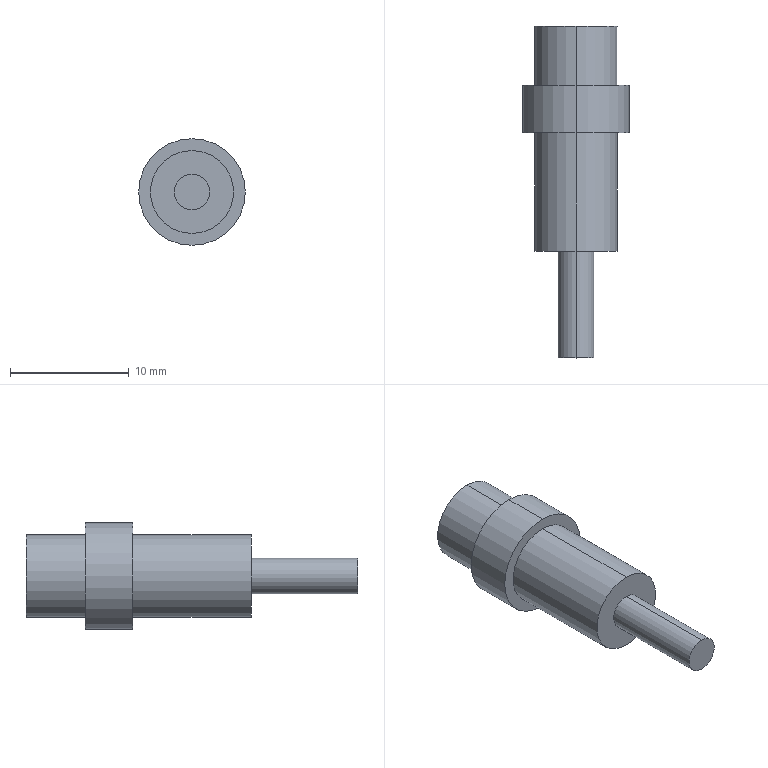Part | SolidWorks | features Revolution 1 | 1 solid | 13 faces | box 9 x 28 x 9 mm | volume 895.354 mm3 | cylinder 8 | plane 5 | commonest cylinder face diameters 7 x4 3 x2 9 x2
STEP:
#1=CARTESIAN_POINT('',(0.,-8.929,-1.5));
#2=VERTEX_POINT('',#1);
#3=CARTESIAN_POINT('',(0.,-8.929,1.5));
#4=VERTEX_POINT('',#3);
#5=CARTESIAN_POINT('',(0.,-8.929,0.));
#6=DIRECTION('',(0.,-1.,0.));
#7=DIRECTION('',(0.,0.,-1.));
#8=AXIS2_PLACEMENT_3D('',#5,#6,#7);
#9=CIRCLE('',#8,1.5);
#10=EDGE_CURVE('',#2,#4,#9,.T.);
#11=ORIENTED_EDGE('',*,*,#10,.T.);
#12=CARTESIAN_POINT('',(0.,-17.929,1.5));
#13=VERTEX_POINT('',#12);
#14=CARTESIAN_POINT('',(0.,0.,1.5));
#15=DIRECTION('',(0.,-1.,0.));
#16=VECTOR('',#15,1000.);
#17=LINE('',#14,#16);
#18=EDGE_CURVE('',#4,#13,#17,.T.);
#19=ORIENTED_EDGE('',*,*,#18,.T.);
#20=CARTESIAN_POINT('',(0.,-17.929,-1.5));
#21=VERTEX_POINT('',#20);
#22=CARTESIAN_POINT('',(0.,-17.929,0.));
#23=DIRECTION('',(0.,-1.,0.));
#24=DIRECTION('',(0.,0.,-1.));
#25=AXIS2_PLACEMENT_3D('',#22,#23,#24);
#26=CIRCLE('',#25,1.5);
#27=EDGE_CURVE('',#21,#13,#26,.T.);
#28=ORIENTED_EDGE('',*,*,#27,.F.);
#29=CARTESIAN_POINT('',(0.,0.,-1.5));
#30=DIRECTION('',(0.,-1.,0.));
#31=VECTOR('',#30,1000.);
#32=LINE('',#29,#31);
#33=EDGE_CURVE('',#2,#21,#32,.T.);
#34=ORIENTED_EDGE('',*,*,#33,.F.);
#35=EDGE_LOOP('',(#11,#19,#28,#34));
#36=FACE_OUTER_BOUND('',#35,.T.);
#37=CARTESIAN_POINT('',(0.,0.,0.));
#38=DIRECTION('',(0.,-1.,0.));
#39=DIRECTION('',(0.,0.,-1.));
#40=AXIS2_PLACEMENT_3D('',#37,#38,#39);
#41=CYLINDRICAL_SURFACE('',#40,1.5);
#42=ADVANCED_FACE('',(#36),#41,.T.);
#43=CARTESIAN_POINT('',(0.,1.071,-3.5));
#44=VERTEX_POINT('',#43);
#45=CARTESIAN_POINT('',(0.,1.071,3.5));
#46=VERTEX_POINT('',#45);
#47=CARTESIAN_POINT('',(0.,1.071,0.));
#48=DIRECTION('',(0.,-1.,0.));
#49=DIRECTION('',(0.,0.,-1.));
#50=AXIS2_PLACEMENT_3D('',#47,#48,#49);
#51=CIRCLE('',#50,3.5);
#52=EDGE_CURVE('',#44,#46,#51,.T.);
#53=ORIENTED_EDGE('',*,*,#52,.T.);
#54=CARTESIAN_POINT('',(0.,-8.929,3.5));
#55=VERTEX_POINT('',#54);
#56=CARTESIAN_POINT('',(0.,0.,3.5));
#57=DIRECTION('',(0.,-1.,0.));
#58=VECTOR('',#57,1000.);
#59=LINE('',#56,#58);
#60=EDGE_CURVE('',#46,#55,#59,.T.);
#61=ORIENTED_EDGE('',*,*,#60,.T.);
#62=CARTESIAN_POINT('',(0.,-8.929,-3.5));
#63=VERTEX_POINT('',#62);
#64=CARTESIAN_POINT('',(0.,-8.929,0.));
#65=DIRECTION('',(0.,-1.,0.));
#66=DIRECTION('',(0.,0.,-1.));
#67=AXIS2_PLACEMENT_3D('',#64,#65,#66);
#68=CIRCLE('',#67,3.5);
#69=EDGE_CURVE('',#63,#55,#68,.T.);
#70=ORIENTED_EDGE('',*,*,#69,.F.);
#71=CARTESIAN_POINT('',(0.,0.,-3.5));
#72=DIRECTION('',(0.,-1.,0.));
#73=VECTOR('',#72,1000.);
#74=LINE('',#71,#73);
#75=EDGE_CURVE('',#44,#63,#74,.T.);
#76=ORIENTED_EDGE('',*,*,#75,.F.);
#77=EDGE_LOOP('',(#53,#61,#70,#76));
#78=FACE_OUTER_BOUND('',#77,.T.);
#79=CARTESIAN_POINT('',(0.,0.,0.));
#80=DIRECTION('',(0.,-1.,0.));
#81=DIRECTION('',(0.,0.,-1.));
#82=AXIS2_PLACEMENT_3D('',#79,#80,#81);
#83=CYLINDRICAL_SURFACE('',#82,3.5);
#84=ADVANCED_FACE('',(#78),#83,.T.);
#85=CARTESIAN_POINT('',(0.,5.071,-4.5));
#86=VERTEX_POINT('',#85);
#87=CARTESIAN_POINT('',(0.,5.071,4.5));
#88=VERTEX_POINT('',#87);
#89=CARTESIAN_POINT('',(0.,5.071,0.));
#90=DIRECTION('',(0.,-1.,0.));
#91=DIRECTION('',(0.,0.,-1.));
#92=AXIS2_PLACEMENT_3D('',#89,#90,#91);
#93=CIRCLE('',#92,4.5);
#94=EDGE_CURVE('',#86,#88,#93,.T.);
#95=ORIENTED_EDGE('',*,*,#94,.T.);
#96=CARTESIAN_POINT('',(0.,1.071,4.5));
#97=VERTEX_POINT('',#96);
#98=CARTESIAN_POINT('',(0.,0.,4.5));
#99=DIRECTION('',(0.,-1.,0.));
#100=VECTOR('',#99,1000.);
#101=LINE('',#98,#100);
#102=EDGE_CURVE('',#88,#97,#101,.T.);
#103=ORIENTED_EDGE('',*,*,#102,.T.);
#104=CARTESIAN_POINT('',(0.,1.071,-4.5));
#105=VERTEX_POINT('',#104);
#106=CARTESIAN_POINT('',(0.,1.071,0.));
#107=DIRECTION('',(0.,-1.,0.));
#108=DIRECTION('',(0.,0.,-1.));
#109=AXIS2_PLACEMENT_3D('',#106,#107,#108);
#110=CIRCLE('',#109,4.5);
#111=EDGE_CURVE('',#105,#97,#110,.T.);
#112=ORIENTED_EDGE('',*,*,#111,.F.);
#113=CARTESIAN_POINT('',(0.,0.,-4.5));
#114=DIRECTION('',(0.,-1.,0.));
#115=VECTOR('',#114,1000.);
#116=LINE('',#113,#115);
#117=EDGE_CURVE('',#86,#105,#116,.T.);
#118=ORIENTED_EDGE('',*,*,#117,.F.);
#119=EDGE_LOOP('',(#95,#103,#112,#118));
#120=FACE_OUTER_BOUND('',#119,.T.);
#121=CARTESIAN_POINT('',(0.,0.,0.));
#122=DIRECTION('',(0.,-1.,0.));
#123=DIRECTION('',(0.,0.,-1.));
#124=AXIS2_PLACEMENT_3D('',#121,#122,#123);
#125=CYLINDRICAL_SURFACE('',#124,4.5);
#126=ADVANCED_FACE('',(#120),#125,.T.);
#127=CARTESIAN_POINT('',(0.,10.071,-3.5));
#128=VERTEX_POINT('',#127);
#129=CARTESIAN_POINT('',(0.,10.071,3.5));
#130=VERTEX_POINT('',#129);
#131=CARTESIAN_POINT('',(0.,10.071,0.));
#132=DIRECTION('',(0.,-1.,0.));
#133=DIRECTION('',(0.,0.,-1.));
#134=AXIS2_PLACEMENT_3D('',#131,#132,#133);
#135=CIRCLE('',#134,3.5);
#136=EDGE_CURVE('',#128,#130,#135,.T.);
#137=ORIENTED_EDGE('',*,*,#136,.T.);
#138=CARTESIAN_POINT('',(0.,5.071,3.5));
#139=VERTEX_POINT('',#138);
#140=CARTESIAN_POINT('',(0.,0.,3.5));
#141=DIRECTION('',(0.,-1.,0.));
#142=VECTOR('',#141,1000.);
#143=LINE('',#140,#142);
#144=EDGE_CURVE('',#130,#139,#143,.T.);
#145=ORIENTED_EDGE('',*,*,#144,.T.);
#146=CARTESIAN_POINT('',(0.,5.071,-3.5));
#147=VERTEX_POINT('',#146);
#148=CARTESIAN_POINT('',(0.,5.071,0.));
#149=DIRECTION('',(0.,-1.,0.));
#150=DIRECTION('',(0.,0.,-1.));
#151=AXIS2_PLACEMENT_3D('',#148,#149,#150);
#152=CIRCLE('',#151,3.5);
#153=EDGE_CURVE('',#147,#139,#152,.T.);
#154=ORIENTED_EDGE('',*,*,#153,.F.);
#155=CARTESIAN_POINT('',(0.,0.,-3.5));
#156=DIRECTION('',(0.,-1.,0.));
#157=VECTOR('',#156,1000.);
#158=LINE('',#155,#157);
#159=EDGE_CURVE('',#128,#147,#158,.T.);
#160=ORIENTED_EDGE('',*,*,#159,.F.);
#161=EDGE_LOOP('',(#137,#145,#154,#160));
#162=FACE_OUTER_BOUND('',#161,.T.);
#163=CARTESIAN_POINT('',(0.,0.,0.));
#164=DIRECTION('',(0.,-1.,0.));
#165=DIRECTION('',(0.,0.,-1.));
#166=AXIS2_PLACEMENT_3D('',#163,#164,#165);
#167=CYLINDRICAL_SURFACE('',#166,3.5);
#168=ADVANCED_FACE('',(#162),#167,.T.);
#169=ORIENTED_EDGE('',*,*,#136,.F.);
#170=CARTESIAN_POINT('',(0.,10.071,0.));
#171=DIRECTION('',(0.,-1.,0.));
#172=DIRECTION('',(0.,0.,-1.));
#173=AXIS2_PLACEMENT_3D('',#170,#171,#172);
#174=CIRCLE('',#173,3.5);
#175=EDGE_CURVE('',#130,#128,#174,.T.);
#176=ORIENTED_EDGE('',*,*,#175,.F.);
#177=EDGE_LOOP('',(#169,#176));
#178=FACE_OUTER_BOUND('',#177,.T.);
#179=CARTESIAN_POINT('',(0.,10.071,0.));
#180=DIRECTION('',(0.,1.,0.));
#181=DIRECTION('',(0.,0.,1.));
#182=AXIS2_PLACEMENT_3D('',#179,#180,#181);
#183=PLANE('',#182);
#184=ADVANCED_FACE('',(#178),#183,.T.);
#185=ORIENTED_EDGE('',*,*,#144,.F.);
#186=ORIENTED_EDGE('',*,*,#175,.T.);
#187=ORIENTED_EDGE('',*,*,#159,.T.);
#188=CARTESIAN_POINT('',(0.,5.071,0.));
#189=DIRECTION('',(0.,-1.,0.));
#190=DIRECTION('',(0.,0.,-1.));
#191=AXIS2_PLACEMENT_3D('',#188,#189,#190);
#192=CIRCLE('',#191,3.5);
#193=EDGE_CURVE('',#139,#147,#192,.T.);
#194=ORIENTED_EDGE('',*,*,#193,.F.);
#195=EDGE_LOOP('',(#185,#186,#187,#194));
#196=FACE_OUTER_BOUND('',#195,.T.);
#197=CARTESIAN_POINT('',(0.,0.,0.));
#198=DIRECTION('',(0.,-1.,0.));
#199=DIRECTION('',(0.,0.,-1.));
#200=AXIS2_PLACEMENT_3D('',#197,#198,#199);
#201=CYLINDRICAL_SURFACE('',#200,3.5);
#202=ADVANCED_FACE('',(#196),#201,.T.);
#203=ORIENTED_EDGE('',*,*,#153,.T.);
#204=ORIENTED_EDGE('',*,*,#193,.T.);
#205=EDGE_LOOP('',(#203,#204));
#206=FACE_BOUND('',#205,.T.);
#207=ORIENTED_EDGE('',*,*,#94,.F.);
#208=CARTESIAN_POINT('',(0.,5.071,0.));
#209=DIRECTION('',(0.,-1.,0.));
#210=DIRECTION('',(0.,0.,-1.));
#211=AXIS2_PLACEMENT_3D('',#208,#209,#210);
#212=CIRCLE('',#211,4.5);
#213=EDGE_CURVE('',#88,#86,#212,.T.);
#214=ORIENTED_EDGE('',*,*,#213,.F.);
#215=EDGE_LOOP('',(#207,#214));
#216=FACE_OUTER_BOUND('',#215,.T.);
#217=CARTESIAN_POINT('',(3.5,5.071,0.));
#218=DIRECTION('',(0.,1.,0.));
#219=DIRECTION('',(0.,0.,1.));
#220=AXIS2_PLACEMENT_3D('',#217,#218,#219);
#221=PLANE('',#220);
#222=ADVANCED_FACE('',(#206,#216),#221,.T.);
#223=ORIENTED_EDGE('',*,*,#102,.F.);
#224=ORIENTED_EDGE('',*,*,#213,.T.);
#225=ORIENTED_EDGE('',*,*,#117,.T.);
#226=CARTESIAN_POINT('',(0.,1.071,0.));
#227=DIRECTION('',(0.,-1.,0.));
#228=DIRECTION('',(0.,0.,-1.));
#229=AXIS2_PLACEMENT_3D('',#226,#227,#228);
#230=CIRCLE('',#229,4.5);
#231=EDGE_CURVE('',#97,#105,#230,.T.);
#232=ORIENTED_EDGE('',*,*,#231,.F.);
#233=EDGE_LOOP('',(#223,#224,#225,#232));
#234=FACE_OUTER_BOUND('',#233,.T.);
#235=CARTESIAN_POINT('',(0.,0.,0.));
#236=DIRECTION('',(0.,-1.,0.));
#237=DIRECTION('',(0.,0.,-1.));
#238=AXIS2_PLACEMENT_3D('',#235,#236,#237);
#239=CYLINDRICAL_SURFACE('',#238,4.5);
#240=ADVANCED_FACE('',(#234),#239,.T.);
#241=ORIENTED_EDGE('',*,*,#111,.T.);
#242=ORIENTED_EDGE('',*,*,#231,.T.);
#243=EDGE_LOOP('',(#241,#242));
#244=FACE_OUTER_BOUND('',#243,.T.);
#245=ORIENTED_EDGE('',*,*,#52,.F.);
#246=CARTESIAN_POINT('',(0.,1.071,0.));
#247=DIRECTION('',(0.,-1.,0.));
#248=DIRECTION('',(0.,0.,-1.));
#249=AXIS2_PLACEMENT_3D('',#246,#247,#248);
#250=CIRCLE('',#249,3.5);
#251=EDGE_CURVE('',#46,#44,#250,.T.);
#252=ORIENTED_EDGE('',*,*,#251,.F.);
#253=EDGE_LOOP('',(#245,#252));
#254=FACE_BOUND('',#253,.T.);
#255=CARTESIAN_POINT('',(4.5,1.071,0.));
#256=DIRECTION('',(0.,-1.,0.));
#257=DIRECTION('',(0.,0.,-1.));
#258=AXIS2_PLACEMENT_3D('',#255,#256,#257);
#259=PLANE('',#258);
#260=ADVANCED_FACE('',(#244,#254),#259,.T.);
#261=ORIENTED_EDGE('',*,*,#60,.F.);
#262=ORIENTED_EDGE('',*,*,#251,.T.);
#263=ORIENTED_EDGE('',*,*,#75,.T.);
#264=CARTESIAN_POINT('',(0.,-8.929,0.));
#265=DIRECTION('',(0.,-1.,0.));
#266=DIRECTION('',(0.,0.,-1.));
#267=AXIS2_PLACEMENT_3D('',#264,#265,#266);
#268=CIRCLE('',#267,3.5);
#269=EDGE_CURVE('',#55,#63,#268,.T.);
#270=ORIENTED_EDGE('',*,*,#269,.F.);
#271=EDGE_LOOP('',(#261,#262,#263,#270));
#272=FACE_OUTER_BOUND('',#271,.T.);
#273=CARTESIAN_POINT('',(0.,0.,0.));
#274=DIRECTION('',(0.,-1.,0.));
#275=DIRECTION('',(0.,0.,-1.));
#276=AXIS2_PLACEMENT_3D('',#273,#274,#275);
#277=CYLINDRICAL_SURFACE('',#276,3.5);
#278=ADVANCED_FACE('',(#272),#277,.T.);
#279=ORIENTED_EDGE('',*,*,#69,.T.);
#280=ORIENTED_EDGE('',*,*,#269,.T.);
#281=EDGE_LOOP('',(#279,#280));
#282=FACE_OUTER_BOUND('',#281,.T.);
#283=ORIENTED_EDGE('',*,*,#10,.F.);
#284=CARTESIAN_POINT('',(0.,-8.929,0.));
#285=DIRECTION('',(0.,-1.,0.));
#286=DIRECTION('',(0.,0.,-1.));
#287=AXIS2_PLACEMENT_3D('',#284,#285,#286);
#288=CIRCLE('',#287,1.5);
#289=EDGE_CURVE('',#4,#2,#288,.T.);
#290=ORIENTED_EDGE('',*,*,#289,.F.);
#291=EDGE_LOOP('',(#283,#290));
#292=FACE_BOUND('',#291,.T.);
#293=CARTESIAN_POINT('',(3.5,-8.929,0.));
#294=DIRECTION('',(0.,-1.,0.));
#295=DIRECTION('',(0.,0.,-1.));
#296=AXIS2_PLACEMENT_3D('',#293,#294,#295);
#297=PLANE('',#296);
#298=ADVANCED_FACE('',(#282,#292),#297,.T.);
#299=ORIENTED_EDGE('',*,*,#18,.F.);
#300=ORIENTED_EDGE('',*,*,#289,.T.);
#301=ORIENTED_EDGE('',*,*,#33,.T.);
#302=CARTESIAN_POINT('',(0.,-17.929,0.));
#303=DIRECTION('',(0.,-1.,0.));
#304=DIRECTION('',(0.,0.,-1.));
#305=AXIS2_PLACEMENT_3D('',#302,#303,#304);
#306=CIRCLE('',#305,1.5);
#307=EDGE_CURVE('',#13,#21,#306,.T.);
#308=ORIENTED_EDGE('',*,*,#307,.F.);
#309=EDGE_LOOP('',(#299,#300,#301,#308));
#310=FACE_OUTER_BOUND('',#309,.T.);
#311=CARTESIAN_POINT('',(0.,0.,0.));
#312=DIRECTION('',(0.,-1.,0.));
#313=DIRECTION('',(0.,0.,-1.));
#314=AXIS2_PLACEMENT_3D('',#311,#312,#313);
#315=CYLINDRICAL_SURFACE('',#314,1.5);
#316=ADVANCED_FACE('',(#310),#315,.T.);
#317=ORIENTED_EDGE('',*,*,#27,.T.);
#318=ORIENTED_EDGE('',*,*,#307,.T.);
#319=EDGE_LOOP('',(#317,#318));
#320=FACE_OUTER_BOUND('',#319,.T.);
#321=CARTESIAN_POINT('',(1.5,-17.929,0.));
#322=DIRECTION('',(0.,-1.,0.));
#323=DIRECTION('',(0.,0.,-1.));
#324=AXIS2_PLACEMENT_3D('',#321,#322,#323);
#325=PLANE('',#324);
#326=ADVANCED_FACE('',(#320),#325,.T.);
#327=CLOSED_SHELL('',(#42,#84,#126,#168,#184,#202,#222,#240,#260,#278,#298,#316,#326));
#328=MANIFOLD_SOLID_BREP('',#327);
#329=CARTESIAN_POINT('',(0.,0.,0.));
#330=DIRECTION('',(0.,0.,1.));
#331=DIRECTION('',(1.,0.,0.));
#332=AXIS2_PLACEMENT_3D('',#329,#330,#331);
#333=(LENGTH_UNIT()NAMED_UNIT(*)SI_UNIT(.MILLI.,.METRE.));
#334=UNCERTAINTY_MEASURE_WITH_UNIT(LENGTH_MEASURE(0.00001),#333,'','');
#335=(NAMED_UNIT(*)PLANE_ANGLE_UNIT()SI_UNIT($,.RADIAN.));
#336=(NAMED_UNIT(*)SI_UNIT($,.STERADIAN.)SOLID_ANGLE_UNIT());
#337=(GEOMETRIC_REPRESENTATION_CONTEXT(3)GLOBAL_UNCERTAINTY_ASSIGNED_CONTEXT((#334))GLOBAL_UNIT_ASSIGNED_CONTEXT((#333,#335,#336))REPRESENTATION_CONTEXT('',''));
#338=ADVANCED_BREP_SHAPE_REPRESENTATION('',(#328,#332),#337);